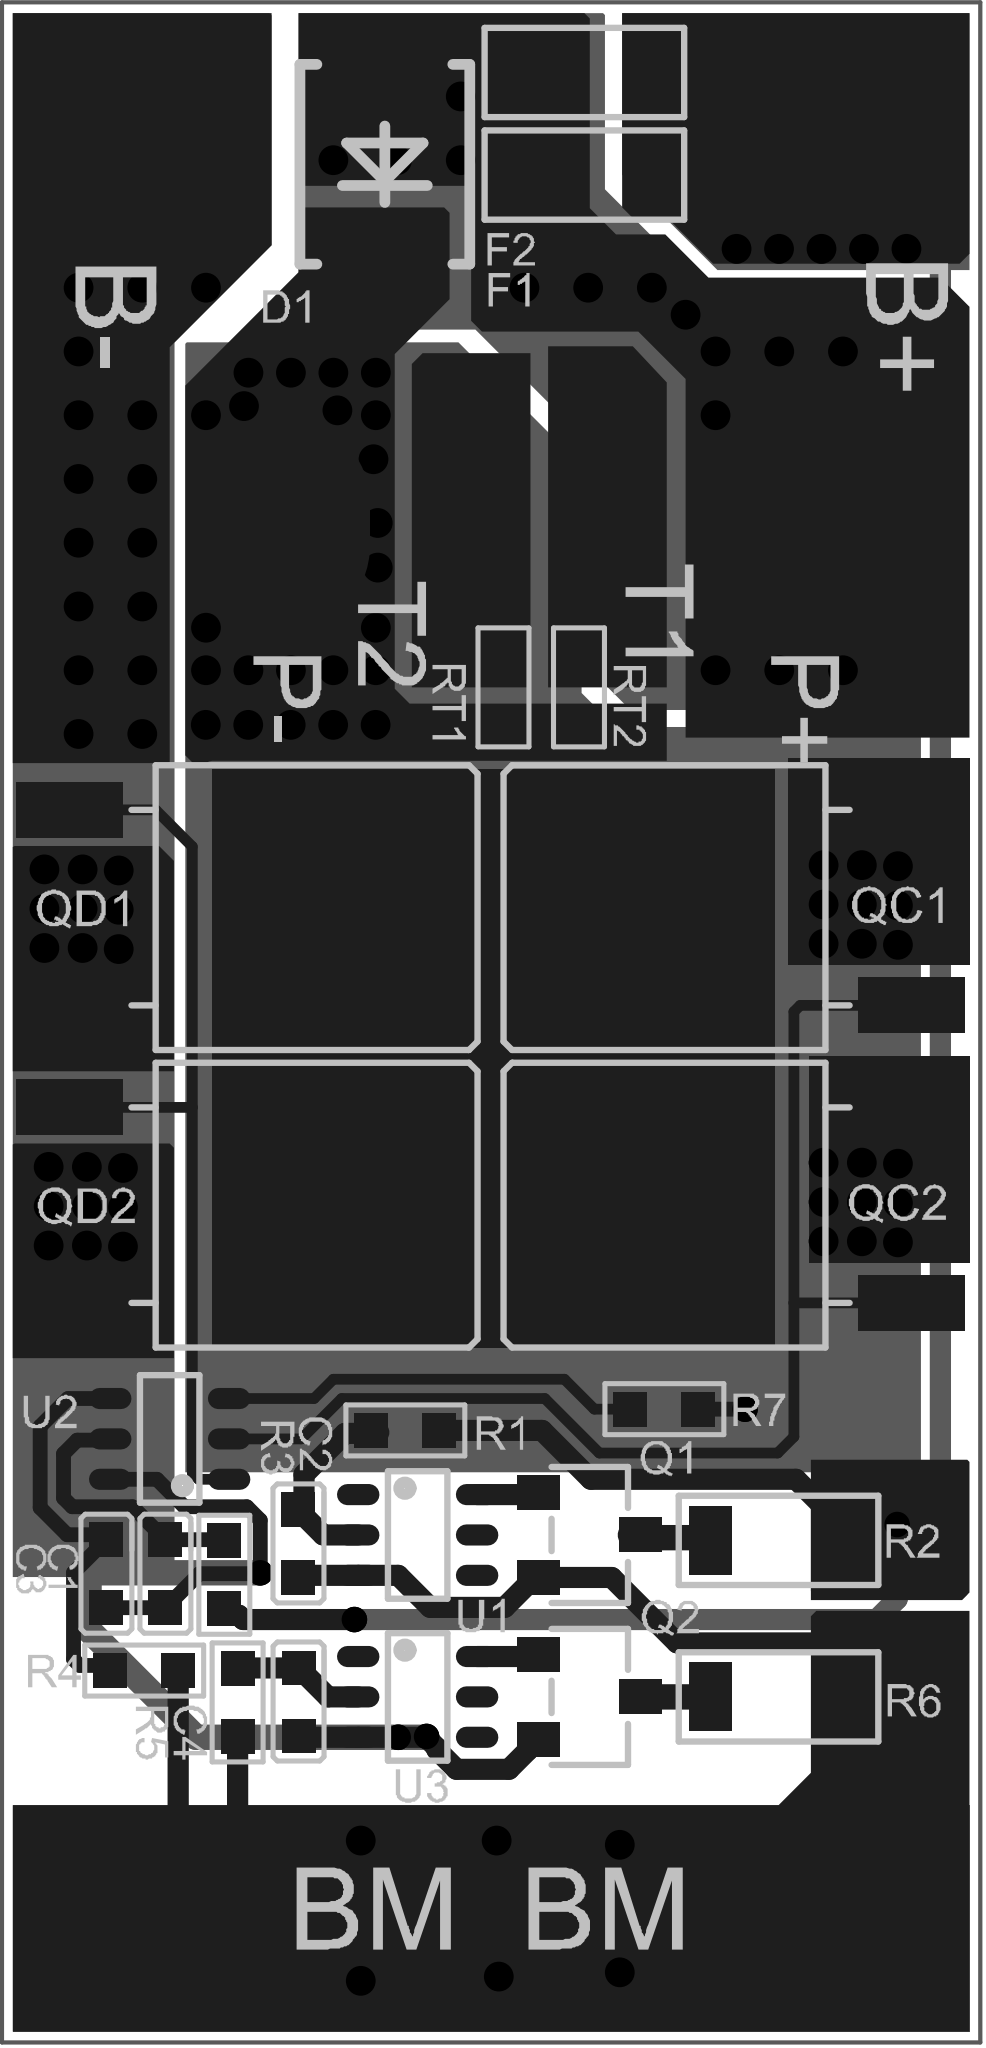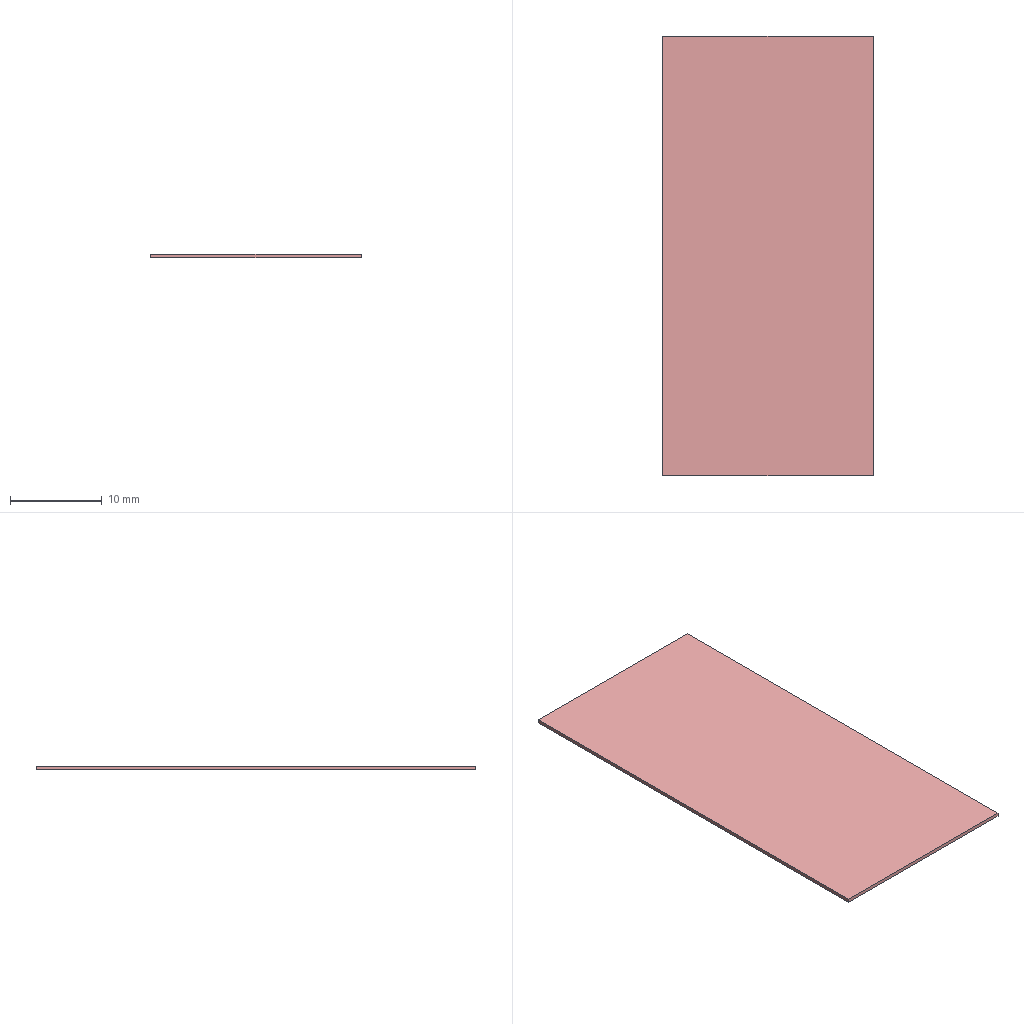Circuit board layout | Altium Designer | box 23 x 48 x 0.4 mm
Layer stack:
# Altium Designer layer stack of  (unit mm; dielectric type: 0 none, 1 core, 2 prepreg, 3 surface material)
index,name,kind,layer,copper_thickness_mm,dielectric_type,dielectric_thickness_mm,dielectric_material,dielectric_constant
0,Top Paste,other,,,,,,
1,Top Overlay,other,,,,,,
2,Top Solder,dielectric,,,3,0.0102,Solder Resist,3.5
3,Top Layer,copper,Top Layer,0.0356,,,,
4,Dielectric 1,dielectric,,,0,0.32,FR-4,4.8
5,Bottom Layer,copper,Bottom Layer,0.0356,,,,
6,Bottom Solder,dielectric,,,3,0.0102,Solder Resist,3.5
7,Bottom Overlay,other,,,,,,
8,Bottom Paste,other,,,,,,
# drill layer pairs: low layer,high layer
drill_pair,Top Layer,Bottom Layer
Part placement:
Designator,Comment,Layer,Footprint,Center-X(mm),Center-Y(mm),Rotation
QD2,N MOS*,TopLayer,TO-252,4.8,-28.3,270
QD1,N MOS*,TopLayer,TO-252,4.8,-21.3,270
QC2,N MOS*,TopLayer,TO-252,18.212,-28.3,90
QC1,N MOS*,TopLayer,TO-252,18.212,-21.3,90
BM,Pad,TopLayer,Pad10X8mm,19.546,-45.04,90
Q2,3400,TopLayer,SOT23-3L,13.843,-39.87,270
Q1,3400,TopLayer,SOT23-3L,13.843,-36.06,270
D1,RS2M,TopLayer,SMB_A_(1+2-),9.017,-3.81,90
U3,CM1010,TopLayer,SOT23-6A,9.79,-39.87,0
U2,S-8252*,TopLayer,SOT23-6A,3.95,-33.8,180
U1,CM1010,TopLayer,SOT23-6A,9.79,-36.06,0
T2,Pad,TopLayer,Pad10X8mm,10.998,-10.977,180
T1,Pad,TopLayer,Pad10X8mm,14.208,-10.977,180
RT2,NC,TopLayer,R0603A,13.589,-16.118,90
RT1,NC,TopLayer,R0603A,11.811,-16.118,90
R7,2K,TopLayer,R0603A,15.6,-33.1,180
R6,100R,TopLayer,R1206A,18.288,-39.87,0
R5,1K,TopLayer,R0603A,5.55,-40,270
R4,470R,TopLayer,R0603A,3.35,-39.25,180
R3,470R,TopLayer,R0603A,5.237,-36.996,90
R2,100R,TopLayer,R1206A,18.288,-36.187,0
R1,1K,TopLayer,R0603A,9.5,-33.6,0
P-,Pad,TopLayer,Pad10X8mm,6.618,-12.286,180
P+,Pad,TopLayer,Pad10X8mm,18.883,-12.286,0
F2,F12F10 32V10A,TopLayer,R1206A,13.716,-1.651,180
F1,F12F10 32V10A,TopLayer,R1206A,13.716,-4.064,180
C4,0.1uF,TopLayer,C0603A,6.985,-39.978,90
C3,0.1uF,TopLayer,C0603A,2.46,-36.971,90
C2,0.1uF,TopLayer,C0603A,6.983,-36.259,90
C1,0.1uF,TopLayer,C0603A,3.85,-36.971,90
BM,Pad,TopLayer,Pad10X8mm,3.338,-45.04,270
B-,Pad,TopLayer,Pad10X8mm,3.338,-2.84,90
B+,Pad,TopLayer,Pad10X8mm,19.546,-2.84,90
Pad and via stacks:
# Altium Designer via and pad stacks of  (unit mm). Each distinct definition once, with the count of objects using it.
# via: kind,start_layer,end_layer,hole_mm,diameter_mm,mode(0 simple;1 top-mid-bottom;2 full stack),diameter_per_layer,count,example_net
# pad: kind,layer,hole_mm,hole_type(0 round;1 square;2 slot),plating,top_size,top_shape(1 round;2 rect;3 octagon;9 rounded rect),mid_size,bottom_size,mode,footprint,size_per_layer,count,example
pad,Top Layer,0,0,plated,1x0.5,1,1x0.5,1x0.5,0,SOT23-6A,,18,U3.4
pad,Top Layer,0,0,plated,6x6,2,6x6,6x6,0,TO-252,,4,QC1.3
pad,Top Layer,0,0,plated,1.3x2.5,2,1.3x2.5,1.3x2.5,0,TO-252,,8,QC1.2
pad,Top Layer,0,0,plated,0.8x0.8,2,0.8x0.8,0.8x0.8,0,R0603A,,14,R7.1
pad,Top Layer,0,0,plated,1x1,1,1x1,1x1,0,,,2,622
pad,Top Layer,0,2,plated,2.1x5,1,2.1x5,2.1x5,0,Pad10X8mm,,2,T1.1
pad,Top Layer,0,0,plated,0.8x0.8,2,0.8x0.8,0.8x0.8,0,C0603A,,8,C1.2
pad,Top Layer,0,0,plated,0.8x1,2,0.8x1,0.8x1,0,SOT23-3L,,6,Q1.1
pad,Top Layer,0,0,plated,1x1.6,2,1x1.6,1x1.6,0,R1206A,,8,R2.1
pad,Top Layer,0,0,plated,2x2.5,2,2x2.5,2x2.5,0,SMB A (1+2-),,2,D1.2
pad,Top Layer,0,2,plated,4.1x5.1,1,4.1x5.1,4.1x5.1,0,Pad10X8mm,,2,P+.1
pad,Top Layer,0,2,plated,5x6,2,5x6,5x6,0,Pad10X8mm,,4,B-.1
pad,Bottom Layer,0,0,plated,4.1x5.1,1,4.1x5.1,4.1x5.1,0,,,2,621
pad,Bottom Layer,0,0,plated,5x6,2,5x6,5x6,0,,,4,620
via,Top Layer,Bottom Layer,0.5,0.7,0,,101,P-
via,Top Layer,Bottom Layer,0.4,0.6,0,,6,P-
Copper pours:
name,layer,net,type(0 solid;1 hatched;2 none)
NONET_L02_P-001,Top Layer,B-,0
NONET_L02_P-001,Top Layer,B-,0
NONET_L02_P-001,Top Layer,P-,0
NONET_L02_P-001,Top Layer,P-,0
NONET_L02_P-001,Top Layer,B-,0
NONET_L02_P-001,Top Layer,B+,0
NONET_L02_P-001,Top Layer,B+,0
NONET_L02_P-001,Top Layer,T1,0
NONET_L02_P-001,Top Layer,T2,0
NONET_L02_P-001,Top Layer,P+,0
NONET_L02_P-001,Top Layer,P-,0
NONET_L02_P-001,Top Layer,NetQC1_3,0
NONET_L02_P-001,Top Layer,BM,0
NONET_L02_P-001,Bottom Layer,P+,0
NONET_L02_P-001,Bottom Layer,B+,0
NONET_L02_P-001,Bottom Layer,P-,0
NONET_L02_P-001,Bottom Layer,B+,0
NONET_L02_P-001,Bottom Layer,B-,0
NONET_L02_P-001,Bottom Layer,BM,0
Design rules, without the lines most boards share:
# Altium Designer design rules of  (exported by Altium Designer, unit mm)
# columns: name | kind | enabled | priority | scope1 | scope2 | descriptor | typed fields (field=value)
Schematic Supply Nets | 41 | enabled | 1 | InNet('P-') | All | Supply Net(s)(InNet('P-')) |
NetAntennae | 56 | enabled | 1 | All | All | Net Antennae (Tolerance=0mm) (All) |
SilkToSilkClearance | 55 | enabled | 1 | All | All | Silk to Silk (Clearance=0mm) (All),(All) |
SilkToSolderMaskClearance | 54 | enabled | 1 | IsPad | All | Silk To Solder Mask (Clearance=0mm) (IsPad),(All) |
MinimumSolderMaskSliver | 53 | enabled | 1 | All | All | Minimum Solder Mask Sliver (Gap=0.254mm) (All),(All) |
HoleToHoleClearance | 52 | enabled | 1 | All | All | Hole To Hole Clearance (Gap=0.254mm) (All),(All) | gap=0.254
DiffPairsRouting | 51 | enabled | 1 | All | All | Differential Pairs Uncoupled Length using the Gap Constraints (Min=0.254mm) (Max=0.254mm) (Prefered=0.254mm)  and Width Constraints (Min=0.381mm) (Max=0.381mm) (Prefered=0.381mm) (All) |
HoleSize | 42 | enabled | 1 | All | All | Hole Size Constraint (Min=0.025mm) (Max=2.54mm) (All) |
Height | 50 | enabled | 1 | All | All | Height Constraint (Min=0mm) (Max=25.4mm) (Prefered=12.7mm) (All) | min_height=0 max_height=25.4
ComponentClearance | 24 | enabled | 1 | All | All | Component Clearance Constraint ( Horizontal Gap = 0.254mm, Vertical Gap = 0.254mm ) (All),(All)  | gap=0.254
SolderMaskExpansion | 13 | enabled | 1 | All | All | Solder Mask Expansion (Expansion =0.102mm) (All) | expansion=0.1016
PasteMaskExpansion | 14 | enabled | 1 | All | All | Paste Mask Expansion (Expansion =0mm) (All) | expansion=0
RoutingVias | 11 | enabled | 1 | All | All | Routing Via (MinHoleWidth=0.711mm) (MaxHoleWidth=0.711mm) (PreferredHoleWidth=0.711mm) (MinWidth=1.27mm) (MaxWidth=1.27mm) (PreferedWidth=1.27mm) (All) | via_min_hole=0.7112 via_max_hole=0.7112 via_preferred_diameter=1.27 via_preferred_hole=0.7112
RoutingCorners | 10 | enabled | 1 | All | All | Routing Corners (Style=45-Degree) (Min Setback=2.54mm) (Max Setback=2.54mm) (All) |
Width | 2 | enabled | 1 | All | All | Width Constraint (Min=0.254mm) (Max=100mm) (Preferred=0.254mm) (All) |
PolygonConnect | 20 | enabled | 1 | All | All | Polygon Connect Rule(Direct Connect )(Conductor Width=0.254mm) (Relief Angle=90 Angle) (Entries=4) (Air Gap Width=0.254mm) (All),(All) | connect_style(0=relief,1=direct,2=none)=1 relief_conductor_width=0.254 relief_entries=4
PlaneClearance | 12 | enabled | 1 | All | All | Power Plane Clearance (Clearance =0.508mm) (All) | clearance=0.508
PlaneConnect | 6 | enabled | 1 | All | All | Power Plane Connect Rule(Relief Connect )(Expansion=0.508mm) (Conductor Width=0.254mm) (Air Gap=0.254mm) (Entries=4) (All) | relief_conductor_width=0.254 relief_entries=4 relief_expansion=0.508
Clearance | 0 | enabled | 1 | All | All | Clearance Constraint (Gap=0.2mm) (All),(All) | gap=0.2